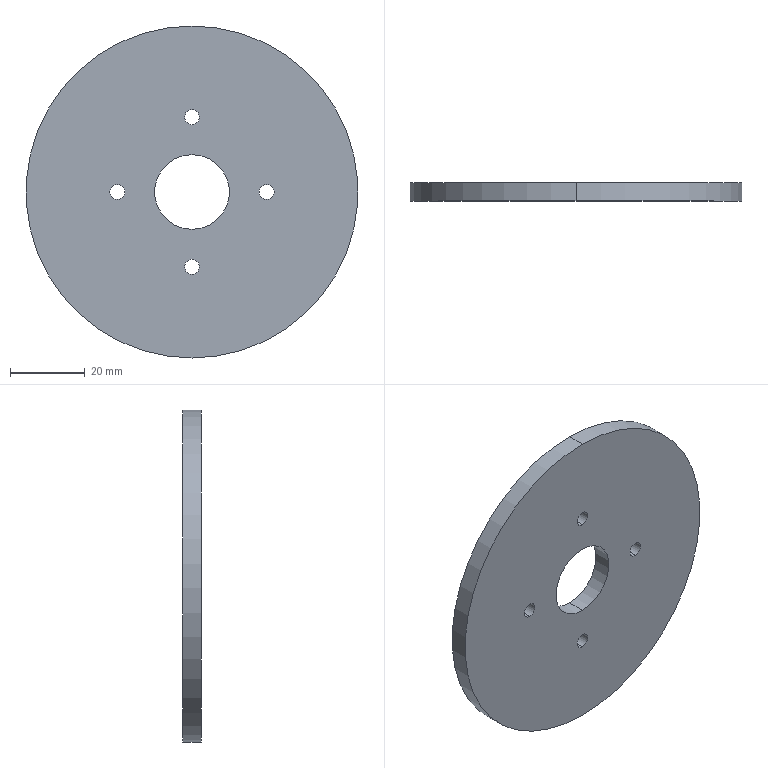Part | STEP file | Guide wheel mechanism revised.sldasm-Part-71 | 1 solid | 34 faces | box 88.8 x 4.9 x 88.8 mm | volume 28486 mm3 | plane 22 | cylinder 12 | commonest cylinder face diameters 4 x8 20 x2 88.8 x2
STEP:
#1=CARTESIAN_POINT('',(-20.,15.1,-2.));
#2=VERTEX_POINT('',#1);
#3=CARTESIAN_POINT('',(-20.,15.1,2.));
#4=VERTEX_POINT('',#3);
#5=CARTESIAN_POINT('',(-20.,15.1,0.));
#6=DIRECTION('',(0.,1.,0.));
#7=DIRECTION('',(0.,0.,-1.));
#8=AXIS2_PLACEMENT_3D('',#5,#6,#7);
#9=CIRCLE('',#8,2.);
#10=EDGE_CURVE('',#2,#4,#9,.T.);
#11=ORIENTED_EDGE('',*,*,#10,.F.);
#12=CARTESIAN_POINT('',(-20.,19.9,-2.));
#13=VERTEX_POINT('',#12);
#14=CARTESIAN_POINT('',(-20.,15.099,-2.));
#15=DIRECTION('',(0.,1.,0.));
#16=VECTOR('',#15,1000.);
#17=LINE('',#14,#16);
#18=EDGE_CURVE('',#2,#13,#17,.T.);
#19=ORIENTED_EDGE('',*,*,#18,.T.);
#20=CARTESIAN_POINT('',(-20.,19.9,2.));
#21=VERTEX_POINT('',#20);
#22=CARTESIAN_POINT('',(-20.,19.9,0.));
#23=DIRECTION('',(0.,1.,0.));
#24=DIRECTION('',(1.,0.,0.));
#25=AXIS2_PLACEMENT_3D('',#22,#23,#24);
#26=CIRCLE('',#25,2.);
#27=EDGE_CURVE('',#13,#21,#26,.T.);
#28=ORIENTED_EDGE('',*,*,#27,.T.);
#29=CARTESIAN_POINT('',(-20.,15.099,2.));
#30=DIRECTION('',(0.,1.,0.));
#31=VECTOR('',#30,1000.);
#32=LINE('',#29,#31);
#33=EDGE_CURVE('',#4,#21,#32,.T.);
#34=ORIENTED_EDGE('',*,*,#33,.F.);
#35=EDGE_LOOP('',(#11,#19,#28,#34));
#36=FACE_OUTER_BOUND('',#35,.T.);
#37=CARTESIAN_POINT('',(-20.,15.099,0.));
#38=DIRECTION('',(0.,1.,0.));
#39=DIRECTION('',(0.,0.,1.));
#40=AXIS2_PLACEMENT_3D('',#37,#38,#39);
#41=CYLINDRICAL_SURFACE('',#40,2.);
#42=ADVANCED_FACE('',(#36),#41,.F.);
#43=CARTESIAN_POINT('',(0.,15.1,18.));
#44=VERTEX_POINT('',#43);
#45=CARTESIAN_POINT('',(0.,15.1,22.));
#46=VERTEX_POINT('',#45);
#47=CARTESIAN_POINT('',(0.,15.1,20.));
#48=DIRECTION('',(0.,1.,0.));
#49=DIRECTION('',(0.,0.,-1.));
#50=AXIS2_PLACEMENT_3D('',#47,#48,#49);
#51=CIRCLE('',#50,2.);
#52=EDGE_CURVE('',#44,#46,#51,.T.);
#53=ORIENTED_EDGE('',*,*,#52,.F.);
#54=CARTESIAN_POINT('',(0.,19.9,18.));
#55=VERTEX_POINT('',#54);
#56=CARTESIAN_POINT('',(0.,15.099,18.));
#57=DIRECTION('',(0.,1.,0.));
#58=VECTOR('',#57,1000.);
#59=LINE('',#56,#58);
#60=EDGE_CURVE('',#44,#55,#59,.T.);
#61=ORIENTED_EDGE('',*,*,#60,.T.);
#62=CARTESIAN_POINT('',(0.,19.9,22.));
#63=VERTEX_POINT('',#62);
#64=CARTESIAN_POINT('',(0.,19.9,20.));
#65=DIRECTION('',(0.,1.,0.));
#66=DIRECTION('',(0.,0.,-1.));
#67=AXIS2_PLACEMENT_3D('',#64,#65,#66);
#68=CIRCLE('',#67,2.);
#69=EDGE_CURVE('',#55,#63,#68,.T.);
#70=ORIENTED_EDGE('',*,*,#69,.T.);
#71=CARTESIAN_POINT('',(0.,15.099,22.));
#72=DIRECTION('',(0.,1.,0.));
#73=VECTOR('',#72,1000.);
#74=LINE('',#71,#73);
#75=EDGE_CURVE('',#46,#63,#74,.T.);
#76=ORIENTED_EDGE('',*,*,#75,.F.);
#77=EDGE_LOOP('',(#53,#61,#70,#76));
#78=FACE_OUTER_BOUND('',#77,.T.);
#79=CARTESIAN_POINT('',(0.,15.099,20.));
#80=DIRECTION('',(0.,1.,0.));
#81=DIRECTION('',(0.,0.,1.));
#82=AXIS2_PLACEMENT_3D('',#79,#80,#81);
#83=CYLINDRICAL_SURFACE('',#82,2.);
#84=ADVANCED_FACE('',(#78),#83,.F.);
#85=CARTESIAN_POINT('',(20.,15.1,-2.));
#86=VERTEX_POINT('',#85);
#87=CARTESIAN_POINT('',(20.,15.1,2.));
#88=VERTEX_POINT('',#87);
#89=CARTESIAN_POINT('',(20.,15.1,0.));
#90=DIRECTION('',(0.,1.,0.));
#91=DIRECTION('',(0.,0.,-1.));
#92=AXIS2_PLACEMENT_3D('',#89,#90,#91);
#93=CIRCLE('',#92,2.);
#94=EDGE_CURVE('',#86,#88,#93,.T.);
#95=ORIENTED_EDGE('',*,*,#94,.F.);
#96=CARTESIAN_POINT('',(20.,19.9,-2.));
#97=VERTEX_POINT('',#96);
#98=CARTESIAN_POINT('',(20.,15.099,-2.));
#99=DIRECTION('',(0.,1.,0.));
#100=VECTOR('',#99,1000.);
#101=LINE('',#98,#100);
#102=EDGE_CURVE('',#86,#97,#101,.T.);
#103=ORIENTED_EDGE('',*,*,#102,.T.);
#104=CARTESIAN_POINT('',(20.,19.9,2.));
#105=VERTEX_POINT('',#104);
#106=CARTESIAN_POINT('',(20.,19.9,0.));
#107=DIRECTION('',(0.,1.,0.));
#108=DIRECTION('',(-1.,0.,0.));
#109=AXIS2_PLACEMENT_3D('',#106,#107,#108);
#110=CIRCLE('',#109,2.);
#111=EDGE_CURVE('',#97,#105,#110,.T.);
#112=ORIENTED_EDGE('',*,*,#111,.T.);
#113=CARTESIAN_POINT('',(20.,15.099,2.));
#114=DIRECTION('',(0.,1.,0.));
#115=VECTOR('',#114,1000.);
#116=LINE('',#113,#115);
#117=EDGE_CURVE('',#88,#105,#116,.T.);
#118=ORIENTED_EDGE('',*,*,#117,.F.);
#119=EDGE_LOOP('',(#95,#103,#112,#118));
#120=FACE_OUTER_BOUND('',#119,.T.);
#121=CARTESIAN_POINT('',(20.,15.099,0.));
#122=DIRECTION('',(0.,1.,0.));
#123=DIRECTION('',(0.,0.,1.));
#124=AXIS2_PLACEMENT_3D('',#121,#122,#123);
#125=CYLINDRICAL_SURFACE('',#124,2.);
#126=ADVANCED_FACE('',(#120),#125,.F.);
#127=CARTESIAN_POINT('',(0.,15.1,-22.));
#128=VERTEX_POINT('',#127);
#129=CARTESIAN_POINT('',(0.,15.1,-18.));
#130=VERTEX_POINT('',#129);
#131=CARTESIAN_POINT('',(0.,15.1,-20.));
#132=DIRECTION('',(0.,1.,0.));
#133=DIRECTION('',(0.,0.,-1.));
#134=AXIS2_PLACEMENT_3D('',#131,#132,#133);
#135=CIRCLE('',#134,2.);
#136=EDGE_CURVE('',#128,#130,#135,.T.);
#137=ORIENTED_EDGE('',*,*,#136,.F.);
#138=CARTESIAN_POINT('',(0.,19.9,-22.));
#139=VERTEX_POINT('',#138);
#140=CARTESIAN_POINT('',(0.,15.099,-22.));
#141=DIRECTION('',(0.,1.,0.));
#142=VECTOR('',#141,1000.);
#143=LINE('',#140,#142);
#144=EDGE_CURVE('',#128,#139,#143,.T.);
#145=ORIENTED_EDGE('',*,*,#144,.T.);
#146=CARTESIAN_POINT('',(0.,19.9,-18.));
#147=VERTEX_POINT('',#146);
#148=CARTESIAN_POINT('',(0.,19.9,-20.));
#149=DIRECTION('',(0.,1.,0.));
#150=DIRECTION('',(0.,0.,1.));
#151=AXIS2_PLACEMENT_3D('',#148,#149,#150);
#152=CIRCLE('',#151,2.);
#153=EDGE_CURVE('',#139,#147,#152,.T.);
#154=ORIENTED_EDGE('',*,*,#153,.T.);
#155=CARTESIAN_POINT('',(0.,15.099,-18.));
#156=DIRECTION('',(0.,1.,0.));
#157=VECTOR('',#156,1000.);
#158=LINE('',#155,#157);
#159=EDGE_CURVE('',#130,#147,#158,.T.);
#160=ORIENTED_EDGE('',*,*,#159,.F.);
#161=EDGE_LOOP('',(#137,#145,#154,#160));
#162=FACE_OUTER_BOUND('',#161,.T.);
#163=CARTESIAN_POINT('',(0.,15.099,-20.));
#164=DIRECTION('',(0.,1.,0.));
#165=DIRECTION('',(0.,0.,1.));
#166=AXIS2_PLACEMENT_3D('',#163,#164,#165);
#167=CYLINDRICAL_SURFACE('',#166,2.);
#168=ADVANCED_FACE('',(#162),#167,.F.);
#169=CARTESIAN_POINT('',(0.,20.,10.));
#170=VERTEX_POINT('',#169);
#171=CARTESIAN_POINT('',(0.,20.,-10.));
#172=VERTEX_POINT('',#171);
#173=CARTESIAN_POINT('',(0.,20.,0.));
#174=DIRECTION('',(0.,-1.,0.));
#175=DIRECTION('',(0.,0.,-1.));
#176=AXIS2_PLACEMENT_3D('',#173,#174,#175);
#177=CIRCLE('',#176,10.);
#178=EDGE_CURVE('',#170,#172,#177,.T.);
#179=ORIENTED_EDGE('',*,*,#178,.F.);
#180=CARTESIAN_POINT('',(0.,15.1,10.));
#181=VERTEX_POINT('',#180);
#182=CARTESIAN_POINT('',(0.,0.,10.));
#183=DIRECTION('',(0.,-1.,0.));
#184=VECTOR('',#183,1000.);
#185=LINE('',#182,#184);
#186=EDGE_CURVE('',#170,#181,#185,.T.);
#187=ORIENTED_EDGE('',*,*,#186,.T.);
#188=CARTESIAN_POINT('',(0.,15.1,-10.));
#189=VERTEX_POINT('',#188);
#190=CARTESIAN_POINT('',(0.,15.1,0.));
#191=DIRECTION('',(0.,-1.,0.));
#192=DIRECTION('',(0.,0.,-1.));
#193=AXIS2_PLACEMENT_3D('',#190,#191,#192);
#194=CIRCLE('',#193,10.);
#195=EDGE_CURVE('',#181,#189,#194,.T.);
#196=ORIENTED_EDGE('',*,*,#195,.T.);
#197=CARTESIAN_POINT('',(0.,0.,-10.));
#198=DIRECTION('',(0.,-1.,0.));
#199=VECTOR('',#198,1000.);
#200=LINE('',#197,#199);
#201=EDGE_CURVE('',#172,#189,#200,.T.);
#202=ORIENTED_EDGE('',*,*,#201,.F.);
#203=EDGE_LOOP('',(#179,#187,#196,#202));
#204=FACE_OUTER_BOUND('',#203,.T.);
#205=CARTESIAN_POINT('',(0.,0.,0.));
#206=DIRECTION('',(0.,-1.,0.));
#207=DIRECTION('',(0.,0.,-1.));
#208=AXIS2_PLACEMENT_3D('',#205,#206,#207);
#209=CYLINDRICAL_SURFACE('',#208,10.);
#210=ADVANCED_FACE('',(#204),#209,.F.);
#211=CARTESIAN_POINT('',(0.,20.,-44.4));
#212=VERTEX_POINT('',#211);
#213=CARTESIAN_POINT('',(0.,20.,44.4));
#214=VERTEX_POINT('',#213);
#215=CARTESIAN_POINT('',(0.,20.,0.));
#216=DIRECTION('',(0.,-1.,0.));
#217=DIRECTION('',(0.,0.,-1.));
#218=AXIS2_PLACEMENT_3D('',#215,#216,#217);
#219=CIRCLE('',#218,44.4);
#220=EDGE_CURVE('',#212,#214,#219,.T.);
#221=ORIENTED_EDGE('',*,*,#220,.T.);
#222=CARTESIAN_POINT('',(0.,15.1,44.4));
#223=VERTEX_POINT('',#222);
#224=CARTESIAN_POINT('',(0.,0.,44.4));
#225=DIRECTION('',(0.,-1.,0.));
#226=VECTOR('',#225,1000.);
#227=LINE('',#224,#226);
#228=EDGE_CURVE('',#214,#223,#227,.T.);
#229=ORIENTED_EDGE('',*,*,#228,.T.);
#230=CARTESIAN_POINT('',(0.,15.1,-44.4));
#231=VERTEX_POINT('',#230);
#232=CARTESIAN_POINT('',(0.,15.1,0.));
#233=DIRECTION('',(0.,-1.,0.));
#234=DIRECTION('',(0.,0.,-1.));
#235=AXIS2_PLACEMENT_3D('',#232,#233,#234);
#236=CIRCLE('',#235,44.4);
#237=EDGE_CURVE('',#231,#223,#236,.T.);
#238=ORIENTED_EDGE('',*,*,#237,.F.);
#239=CARTESIAN_POINT('',(0.,0.,-44.4));
#240=DIRECTION('',(0.,-1.,0.));
#241=VECTOR('',#240,1000.);
#242=LINE('',#239,#241);
#243=EDGE_CURVE('',#212,#231,#242,.T.);
#244=ORIENTED_EDGE('',*,*,#243,.F.);
#245=EDGE_LOOP('',(#221,#229,#238,#244));
#246=FACE_OUTER_BOUND('',#245,.T.);
#247=CARTESIAN_POINT('',(0.,0.,0.));
#248=DIRECTION('',(0.,-1.,0.));
#249=DIRECTION('',(0.,0.,-1.));
#250=AXIS2_PLACEMENT_3D('',#247,#248,#249);
#251=CYLINDRICAL_SURFACE('',#250,44.4);
#252=ADVANCED_FACE('',(#246),#251,.T.);
#253=ORIENTED_EDGE('',*,*,#228,.F.);
#254=CARTESIAN_POINT('',(0.,20.,0.));
#255=DIRECTION('',(0.,-1.,0.));
#256=DIRECTION('',(0.,0.,-1.));
#257=AXIS2_PLACEMENT_3D('',#254,#255,#256);
#258=CIRCLE('',#257,44.4);
#259=EDGE_CURVE('',#214,#212,#258,.T.);
#260=ORIENTED_EDGE('',*,*,#259,.T.);
#261=ORIENTED_EDGE('',*,*,#243,.T.);
#262=CARTESIAN_POINT('',(0.,15.1,0.));
#263=DIRECTION('',(0.,-1.,0.));
#264=DIRECTION('',(0.,0.,-1.));
#265=AXIS2_PLACEMENT_3D('',#262,#263,#264);
#266=CIRCLE('',#265,44.4);
#267=EDGE_CURVE('',#223,#231,#266,.T.);
#268=ORIENTED_EDGE('',*,*,#267,.F.);
#269=EDGE_LOOP('',(#253,#260,#261,#268));
#270=FACE_OUTER_BOUND('',#269,.T.);
#271=CARTESIAN_POINT('',(0.,0.,0.));
#272=DIRECTION('',(0.,-1.,0.));
#273=DIRECTION('',(0.,0.,-1.));
#274=AXIS2_PLACEMENT_3D('',#271,#272,#273);
#275=CYLINDRICAL_SURFACE('',#274,44.4);
#276=ADVANCED_FACE('',(#270),#275,.T.);
#277=CARTESIAN_POINT('',(-35.,20.,5.));
#278=VERTEX_POINT('',#277);
#279=CARTESIAN_POINT('',(-15.,20.,5.));
#280=VERTEX_POINT('',#279);
#281=CARTESIAN_POINT('',(-35.,20.,5.));
#282=DIRECTION('',(1.,0.,0.));
#283=VECTOR('',#282,1000.);
#284=LINE('',#281,#283);
#285=EDGE_CURVE('',#278,#280,#284,.T.);
#286=ORIENTED_EDGE('',*,*,#285,.F.);
#287=CARTESIAN_POINT('',(-35.,20.,-5.));
#288=VERTEX_POINT('',#287);
#289=CARTESIAN_POINT('',(-35.,20.,5.));
#290=DIRECTION('',(0.,0.,1.));
#291=VECTOR('',#290,1000.);
#292=LINE('',#289,#291);
#293=EDGE_CURVE('',#288,#278,#292,.T.);
#294=ORIENTED_EDGE('',*,*,#293,.F.);
#295=CARTESIAN_POINT('',(-15.,20.,-5.));
#296=VERTEX_POINT('',#295);
#297=CARTESIAN_POINT('',(-35.,20.,-5.));
#298=DIRECTION('',(-1.,0.,0.));
#299=VECTOR('',#298,1000.);
#300=LINE('',#297,#299);
#301=EDGE_CURVE('',#296,#288,#300,.T.);
#302=ORIENTED_EDGE('',*,*,#301,.F.);
#303=CARTESIAN_POINT('',(-15.,20.,5.));
#304=DIRECTION('',(0.,0.,-1.));
#305=VECTOR('',#304,1000.);
#306=LINE('',#303,#305);
#307=EDGE_CURVE('',#280,#296,#306,.T.);
#308=ORIENTED_EDGE('',*,*,#307,.F.);
#309=EDGE_LOOP('',(#286,#294,#302,#308));
#310=FACE_BOUND('',#309,.T.);
#311=CARTESIAN_POINT('',(5.,20.,35.));
#312=VERTEX_POINT('',#311);
#313=CARTESIAN_POINT('',(5.,20.,15.));
#314=VERTEX_POINT('',#313);
#315=CARTESIAN_POINT('',(5.,20.,35.));
#316=DIRECTION('',(0.,0.,-1.));
#317=VECTOR('',#316,1000.);
#318=LINE('',#315,#317);
#319=EDGE_CURVE('',#312,#314,#318,.T.);
#320=ORIENTED_EDGE('',*,*,#319,.F.);
#321=CARTESIAN_POINT('',(-5.,20.,35.));
#322=VERTEX_POINT('',#321);
#323=CARTESIAN_POINT('',(5.,20.,35.));
#324=DIRECTION('',(1.,0.,0.));
#325=VECTOR('',#324,1000.);
#326=LINE('',#323,#325);
#327=EDGE_CURVE('',#322,#312,#326,.T.);
#328=ORIENTED_EDGE('',*,*,#327,.F.);
#329=CARTESIAN_POINT('',(-5.,20.,15.));
#330=VERTEX_POINT('',#329);
#331=CARTESIAN_POINT('',(-5.,20.,35.));
#332=DIRECTION('',(0.,0.,1.));
#333=VECTOR('',#332,1000.);
#334=LINE('',#331,#333);
#335=EDGE_CURVE('',#330,#322,#334,.T.);
#336=ORIENTED_EDGE('',*,*,#335,.F.);
#337=CARTESIAN_POINT('',(5.,20.,15.));
#338=DIRECTION('',(-1.,0.,0.));
#339=VECTOR('',#338,1000.);
#340=LINE('',#337,#339);
#341=EDGE_CURVE('',#314,#330,#340,.T.);
#342=ORIENTED_EDGE('',*,*,#341,.F.);
#343=EDGE_LOOP('',(#320,#328,#336,#342));
#344=FACE_BOUND('',#343,.T.);
#345=CARTESIAN_POINT('',(35.,20.,-5.));
#346=VERTEX_POINT('',#345);
#347=CARTESIAN_POINT('',(15.,20.,-5.));
#348=VERTEX_POINT('',#347);
#349=CARTESIAN_POINT('',(35.,20.,-5.));
#350=DIRECTION('',(-1.,0.,0.));
#351=VECTOR('',#350,1000.);
#352=LINE('',#349,#351);
#353=EDGE_CURVE('',#346,#348,#352,.T.);
#354=ORIENTED_EDGE('',*,*,#353,.F.);
#355=CARTESIAN_POINT('',(35.,20.,5.));
#356=VERTEX_POINT('',#355);
#357=CARTESIAN_POINT('',(35.,20.,-5.));
#358=DIRECTION('',(0.,0.,-1.));
#359=VECTOR('',#358,1000.);
#360=LINE('',#357,#359);
#361=EDGE_CURVE('',#356,#346,#360,.T.);
#362=ORIENTED_EDGE('',*,*,#361,.F.);
#363=CARTESIAN_POINT('',(15.,20.,5.));
#364=VERTEX_POINT('',#363);
#365=CARTESIAN_POINT('',(35.,20.,5.));
#366=DIRECTION('',(1.,0.,0.));
#367=VECTOR('',#366,1000.);
#368=LINE('',#365,#367);
#369=EDGE_CURVE('',#364,#356,#368,.T.);
#370=ORIENTED_EDGE('',*,*,#369,.F.);
#371=CARTESIAN_POINT('',(15.,20.,-5.));
#372=DIRECTION('',(0.,0.,1.));
#373=VECTOR('',#372,1000.);
#374=LINE('',#371,#373);
#375=EDGE_CURVE('',#348,#364,#374,.T.);
#376=ORIENTED_EDGE('',*,*,#375,.F.);
#377=EDGE_LOOP('',(#354,#362,#370,#376));
#378=FACE_BOUND('',#377,.T.);
#379=CARTESIAN_POINT('',(-5.,20.,-35.));
#380=VERTEX_POINT('',#379);
#381=CARTESIAN_POINT('',(-5.,20.,-15.));
#382=VERTEX_POINT('',#381);
#383=CARTESIAN_POINT('',(-5.,20.,-35.));
#384=DIRECTION('',(0.,0.,1.));
#385=VECTOR('',#384,1000.);
#386=LINE('',#383,#385);
#387=EDGE_CURVE('',#380,#382,#386,.T.);
#388=ORIENTED_EDGE('',*,*,#387,.F.);
#389=CARTESIAN_POINT('',(5.,20.,-35.));
#390=VERTEX_POINT('',#389);
#391=CARTESIAN_POINT('',(-5.,20.,-35.));
#392=DIRECTION('',(-1.,0.,0.));
#393=VECTOR('',#392,1000.);
#394=LINE('',#391,#393);
#395=EDGE_CURVE('',#390,#380,#394,.T.);
#396=ORIENTED_EDGE('',*,*,#395,.F.);
#397=CARTESIAN_POINT('',(5.,20.,-15.));
#398=VERTEX_POINT('',#397);
#399=CARTESIAN_POINT('',(5.,20.,-35.));
#400=DIRECTION('',(0.,0.,-1.));
#401=VECTOR('',#400,1000.);
#402=LINE('',#399,#401);
#403=EDGE_CURVE('',#398,#390,#402,.T.);
#404=ORIENTED_EDGE('',*,*,#403,.F.);
#405=CARTESIAN_POINT('',(-5.,20.,-15.));
#406=DIRECTION('',(1.,0.,0.));
#407=VECTOR('',#406,1000.);
#408=LINE('',#405,#407);
#409=EDGE_CURVE('',#382,#398,#408,.T.);
#410=ORIENTED_EDGE('',*,*,#409,.F.);
#411=EDGE_LOOP('',(#388,#396,#404,#410));
#412=FACE_BOUND('',#411,.T.);
#413=CARTESIAN_POINT('',(0.,20.,0.));
#414=DIRECTION('',(0.,-1.,0.));
#415=DIRECTION('',(0.,0.,-1.));
#416=AXIS2_PLACEMENT_3D('',#413,#414,#415);
#417=CIRCLE('',#416,10.);
#418=EDGE_CURVE('',#172,#170,#417,.T.);
#419=ORIENTED_EDGE('',*,*,#418,.T.);
#420=ORIENTED_EDGE('',*,*,#178,.T.);
#421=EDGE_LOOP('',(#419,#420));
#422=FACE_BOUND('',#421,.T.);
#423=ORIENTED_EDGE('',*,*,#220,.F.);
#424=ORIENTED_EDGE('',*,*,#259,.F.);
#425=EDGE_LOOP('',(#423,#424));
#426=FACE_OUTER_BOUND('',#425,.T.);
#427=CARTESIAN_POINT('',(44.4,20.,0.));
#428=DIRECTION('',(0.,1.,0.));
#429=DIRECTION('',(0.,0.,1.));
#430=AXIS2_PLACEMENT_3D('',#427,#428,#429);
#431=PLANE('',#430);
#432=ADVANCED_FACE('',(#310,#344,#378,#412,#422,#426),#431,.T.);
#433=ORIENTED_EDGE('',*,*,#186,.F.);
#434=ORIENTED_EDGE('',*,*,#418,.F.);
#435=ORIENTED_EDGE('',*,*,#201,.T.);
#436=CARTESIAN_POINT('',(0.,15.1,0.));
#437=DIRECTION('',(0.,-1.,0.));
#438=DIRECTION('',(0.,0.,-1.));
#439=AXIS2_PLACEMENT_3D('',#436,#437,#438);
#440=CIRCLE('',#439,10.);
#441=EDGE_CURVE('',#189,#181,#440,.T.);
#442=ORIENTED_EDGE('',*,*,#441,.T.);
#443=EDGE_LOOP('',(#433,#434,#435,#442));
#444=FACE_OUTER_BOUND('',#443,.T.);
#445=CARTESIAN_POINT('',(0.,0.,0.));
#446=DIRECTION('',(0.,-1.,0.));
#447=DIRECTION('',(0.,0.,-1.));
#448=AXIS2_PLACEMENT_3D('',#445,#446,#447);
#449=CYLINDRICAL_SURFACE('',#448,10.);
#450=ADVANCED_FACE('',(#444),#449,.F.);
#451=CARTESIAN_POINT('',(-20.,15.1,0.));
#452=DIRECTION('',(0.,1.,0.));
#453=DIRECTION('',(0.,0.,-1.));
#454=AXIS2_PLACEMENT_3D('',#451,#452,#453);
#455=CIRCLE('',#454,2.);
#456=EDGE_CURVE('',#4,#2,#455,.T.);
#457=ORIENTED_EDGE('',*,*,#456,.T.);
#458=ORIENTED_EDGE('',*,*,#10,.T.);
#459=EDGE_LOOP('',(#457,#458));
#460=FACE_BOUND('',#459,.T.);
#461=CARTESIAN_POINT('',(0.,15.1,20.));
#462=DIRECTION('',(0.,1.,0.));
#463=DIRECTION('',(0.,0.,-1.));
#464=AXIS2_PLACEMENT_3D('',#461,#462,#463);
#465=CIRCLE('',#464,2.);
#466=EDGE_CURVE('',#46,#44,#465,.T.);
#467=ORIENTED_EDGE('',*,*,#466,.T.);
#468=ORIENTED_EDGE('',*,*,#52,.T.);
#469=EDGE_LOOP('',(#467,#468));
#470=FACE_BOUND('',#469,.T.);
#471=CARTESIAN_POINT('',(20.,15.1,0.));
#472=DIRECTION('',(0.,1.,0.));
#473=DIRECTION('',(0.,0.,-1.));
#474=AXIS2_PLACEMENT_3D('',#471,#472,#473);
#475=CIRCLE('',#474,2.);
#476=EDGE_CURVE('',#88,#86,#475,.T.);
#477=ORIENTED_EDGE('',*,*,#476,.T.);
#478=ORIENTED_EDGE('',*,*,#94,.T.);
#479=EDGE_LOOP('',(#477,#478));
#480=FACE_BOUND('',#479,.T.);
#481=CARTESIAN_POINT('',(0.,15.1,-20.));
#482=DIRECTION('',(0.,1.,0.));
#483=DIRECTION('',(0.,0.,-1.));
#484=AXIS2_PLACEMENT_3D('',#481,#482,#483);
#485=CIRCLE('',#484,2.);
#486=EDGE_CURVE('',#130,#128,#485,.T.);
#487=ORIENTED_EDGE('',*,*,#486,.T.);
#488=ORIENTED_EDGE('',*,*,#136,.T.);
#489=EDGE_LOOP('',(#487,#488));
#490=FACE_BOUND('',#489,.T.);
#491=ORIENTED_EDGE('',*,*,#237,.T.);
#492=ORIENTED_EDGE('',*,*,#267,.T.);
#493=EDGE_LOOP('',(#491,#492));
#494=FACE_OUTER_BOUND('',#493,.T.);
#495=ORIENTED_EDGE('',*,*,#441,.F.);
#496=ORIENTED_EDGE('',*,*,#195,.F.);
#497=EDGE_LOOP('',(#495,#496));
#498=FACE_BOUND('',#497,.T.);
#499=CARTESIAN_POINT('',(10.,15.1,0.));
#500=DIRECTION('',(0.,-1.,0.));
#501=DIRECTION('',(0.,0.,-1.));
#502=AXIS2_PLACEMENT_3D('',#499,#500,#501);
#503=PLANE('',#502);
#504=ADVANCED_FACE('',(#460,#470,#480,#490,#494,#498),#503,.T.);
#505=ORIENTED_EDGE('',*,*,#387,.T.);
#506=CARTESIAN_POINT('',(-5.,19.9,-15.));
#507=VERTEX_POINT('',#506);
#508=CARTESIAN_POINT('',(-5.,19.9,-15.));
#509=DIRECTION('',(0.,1.,0.));
#510=VECTOR('',#509,1000.);
#511=LINE('',#508,#510);
#512=EDGE_CURVE('',#507,#382,#511,.T.);
#513=ORIENTED_EDGE('',*,*,#512,.F.);
#514=CARTESIAN_POINT('',(-5.,19.9,-35.));
#515=VERTEX_POINT('',#514);
#516=CARTESIAN_POINT('',(-5.,19.9,-35.));
#517=DIRECTION('',(0.,0.,1.));
#518=VECTOR('',#517,1000.);
#519=LINE('',#516,#518);
#520=EDGE_CURVE('',#515,#507,#519,.T.);
#521=ORIENTED_EDGE('',*,*,#520,.F.);
#522=CARTESIAN_POINT('',(-5.,19.9,-35.));
#523=DIRECTION('',(0.,1.,0.));
#524=VECTOR('',#523,1000.);
#525=LINE('',#522,#524);
#526=EDGE_CURVE('',#515,#380,#525,.T.);
#527=ORIENTED_EDGE('',*,*,#526,.T.);
#528=EDGE_LOOP('',(#505,#513,#521,#527));
#529=FACE_OUTER_BOUND('',#528,.T.);
#530=CARTESIAN_POINT('',(-5.,19.9,-35.));
#531=DIRECTION('',(-1.,0.,0.));
#532=DIRECTION('',(0.,0.,1.));
#533=AXIS2_PLACEMENT_3D('',#530,#531,#532);
#534=PLANE('',#533);
#535=ADVANCED_FACE('',(#529),#534,.F.);
#536=ORIENTED_EDGE('',*,*,#395,.T.);
#537=ORIENTED_EDGE('',*,*,#526,.F.);
#538=CARTESIAN_POINT('',(5.,19.9,-35.));
#539=VERTEX_POINT('',#538);
#540=CARTESIAN_POINT('',(-5.,19.9,-35.));
#541=DIRECTION('',(-1.,0.,0.));
#542=VECTOR('',#541,1000.);
#543=LINE('',#540,#542);
#544=EDGE_CURVE('',#539,#515,#543,.T.);
#545=ORIENTED_EDGE('',*,*,#544,.F.);
#546=CARTESIAN_POINT('',(5.,19.9,-35.));
#547=DIRECTION('',(0.,1.,0.));
#548=VECTOR('',#547,1000.);
#549=LINE('',#546,#548);
#550=EDGE_CURVE('',#539,#390,#549,.T.);
#551=ORIENTED_EDGE('',*,*,#550,.T.);
#552=EDGE_LOOP('',(#536,#537,#545,#551));
#553=FACE_OUTER_BOUND('',#552,.T.);
#554=CARTESIAN_POINT('',(-5.,19.9,-35.));
#555=DIRECTION('',(0.,0.,-1.));
#556=DIRECTION('',(-1.,0.,0.));
#557=AXIS2_PLACEMENT_3D('',#554,#555,#556);
#558=PLANE('',#557);
#559=ADVANCED_FACE('',(#553),#558,.F.);
#560=ORIENTED_EDGE('',*,*,#403,.T.);
#561=ORIENTED_EDGE('',*,*,#550,.F.);
#562=CARTESIAN_POINT('',(5.,19.9,-15.));
#563=VERTEX_POINT('',#562);
#564=CARTESIAN_POINT('',(5.,19.9,-35.));
#565=DIRECTION('',(0.,0.,-1.));
#566=VECTOR('',#565,1000.);
#567=LINE('',#564,#566);
#568=EDGE_CURVE('',#563,#539,#567,.T.);
#569=ORIENTED_EDGE('',*,*,#568,.F.);
#570=CARTESIAN_POINT('',(5.,19.9,-15.));
#571=DIRECTION('',(0.,1.,0.));
#572=VECTOR('',#571,1000.);
#573=LINE('',#570,#572);
#574=EDGE_CURVE('',#563,#398,#573,.T.);
#575=ORIENTED_EDGE('',*,*,#574,.T.);
#576=EDGE_LOOP('',(#560,#561,#569,#575));
#577=FACE_OUTER_BOUND('',#576,.T.);
#578=CARTESIAN_POINT('',(5.,19.9,-35.));
#579=DIRECTION('',(1.,0.,0.));
#580=DIRECTION('',(0.,0.,-1.));
#581=AXIS2_PLACEMENT_3D('',#578,#579,#580);
#582=PLANE('',#581);
#583=ADVANCED_FACE('',(#577),#582,.F.);
#584=ORIENTED_EDGE('',*,*,#409,.T.);
#585=ORIENTED_EDGE('',*,*,#574,.F.);
#586=CARTESIAN_POINT('',(-5.,19.9,-15.));
#587=DIRECTION('',(1.,0.,0.));
#588=VECTOR('',#587,1000.);
#589=LINE('',#586,#588);
#590=EDGE_CURVE('',#507,#563,#589,.T.);
#591=ORIENTED_EDGE('',*,*,#590,.F.);
#592=ORIENTED_EDGE('',*,*,#512,.T.);
#593=EDGE_LOOP('',(#584,#585,#591,#592));
#594=FACE_OUTER_BOUND('',#593,.T.);
#595=CARTESIAN_POINT('',(-5.,19.9,-15.));
#596=DIRECTION('',(0.,0.,1.));
#597=DIRECTION('',(1.,0.,0.));
#598=AXIS2_PLACEMENT_3D('',#595,#596,#597);
#599=PLANE('',#598);
#600=ADVANCED_FACE('',(#594),#599,.F.);
#601=CARTESIAN_POINT('',(0.,19.9,-20.));
#602=DIRECTION('',(0.,1.,0.));
#603=DIRECTION('',(0.,0.,1.));
#604=AXIS2_PLACEMENT_3D('',#601,#602,#603);
#605=CIRCLE('',#604,2.);
#606=EDGE_CURVE('',#147,#139,#605,.T.);
#607=ORIENTED_EDGE('',*,*,#606,.F.);
#608=ORIENTED_EDGE('',*,*,#153,.F.);
#609=EDGE_LOOP('',(#607,#608));
#610=FACE_BOUND('',#609,.T.);
#611=ORIENTED_EDGE('',*,*,#520,.T.);
#612=ORIENTED_EDGE('',*,*,#590,.T.);
#613=ORIENTED_EDGE('',*,*,#568,.T.);
#614=ORIENTED_EDGE('',*,*,#544,.T.);
#615=EDGE_LOOP('',(#611,#612,#613,#614));
#616=FACE_OUTER_BOUND('',#615,.T.);
#617=CARTESIAN_POINT('',(0.,19.9,0.));
#618=DIRECTION('',(0.,1.,0.));
#619=DIRECTION('',(0.,0.,1.));
#620=AXIS2_PLACEMENT_3D('',#617,#618,#619);
#621=PLANE('',#620);
#622=ADVANCED_FACE('',(#610,#616),#621,.T.);
#623=ORIENTED_EDGE('',*,*,#144,.F.);
#624=ORIENTED_EDGE('',*,*,#486,.F.);
#625=ORIENTED_EDGE('',*,*,#159,.T.);
#626=ORIENTED_EDGE('',*,*,#606,.T.);
#627=EDGE_LOOP('',(#623,#624,#625,#626));
#628=FACE_OUTER_BOUND('',#627,.T.);
#629=CARTESIAN_POINT('',(0.,15.099,-20.));
#630=DIRECTION('',(0.,1.,0.));
#631=DIRECTION('',(0.,0.,1.));
#632=AXIS2_PLACEMENT_3D('',#629,#630,#631);
#633=CYLINDRICAL_SURFACE('',#632,2.);
#634=ADVANCED_FACE('',(#628),#633,.F.);
#635=ORIENTED_EDGE('',*,*,#353,.T.);
#636=CARTESIAN_POINT('',(15.,19.9,-5.));
#637=VERTEX_POINT('',#636);
#638=CARTESIAN_POINT('',(15.,19.9,-5.));
#639=DIRECTION('',(0.,1.,0.));
#640=VECTOR('',#639,1000.);
#641=LINE('',#638,#640);
#642=EDGE_CURVE('',#637,#348,#641,.T.);
#643=ORIENTED_EDGE('',*,*,#642,.F.);
#644=CARTESIAN_POINT('',(35.,19.9,-5.));
#645=VERTEX_POINT('',#644);
#646=CARTESIAN_POINT('',(35.,19.9,-5.));
#647=DIRECTION('',(-1.,0.,0.));
#648=VECTOR('',#647,1000.);
#649=LINE('',#646,#648);
#650=EDGE_CURVE('',#645,#637,#649,.T.);
#651=ORIENTED_EDGE('',*,*,#650,.F.);
#652=CARTESIAN_POINT('',(35.,19.9,-5.));
#653=DIRECTION('',(0.,1.,0.));
#654=VECTOR('',#653,1000.);
#655=LINE('',#652,#654);
#656=EDGE_CURVE('',#645,#346,#655,.T.);
#657=ORIENTED_EDGE('',*,*,#656,.T.);
#658=EDGE_LOOP('',(#635,#643,#651,#657));
#659=FACE_OUTER_BOUND('',#658,.T.);
#660=CARTESIAN_POINT('',(35.,19.9,-5.));
#661=DIRECTION('',(0.,0.,-1.));
#662=DIRECTION('',(-1.,0.,0.));
#663=AXIS2_PLACEMENT_3D('',#660,#661,#662);
#664=PLANE('',#663);
#665=ADVANCED_FACE('',(#659),#664,.F.);
#666=ORIENTED_EDGE('',*,*,#361,.T.);
#667=ORIENTED_EDGE('',*,*,#656,.F.);
#668=CARTESIAN_POINT('',(35.,19.9,5.));
#669=VERTEX_POINT('',#668);
#670=CARTESIAN_POINT('',(35.,19.9,-5.));
#671=DIRECTION('',(0.,0.,-1.));
#672=VECTOR('',#671,1000.);
#673=LINE('',#670,#672);
#674=EDGE_CURVE('',#669,#645,#673,.T.);
#675=ORIENTED_EDGE('',*,*,#674,.F.);
#676=CARTESIAN_POINT('',(35.,19.9,5.));
#677=DIRECTION('',(0.,1.,0.));
#678=VECTOR('',#677,1000.);
#679=LINE('',#676,#678);
#680=EDGE_CURVE('',#669,#356,#679,.T.);
#681=ORIENTED_EDGE('',*,*,#680,.T.);
#682=EDGE_LOOP('',(#666,#667,#675,#681));
#683=FACE_OUTER_BOUND('',#682,.T.);
#684=CARTESIAN_POINT('',(35.,19.9,-5.));
#685=DIRECTION('',(1.,0.,0.));
#686=DIRECTION('',(0.,0.,-1.));
#687=AXIS2_PLACEMENT_3D('',#684,#685,#686);
#688=PLANE('',#687);
#689=ADVANCED_FACE('',(#683),#688,.F.);
#690=ORIENTED_EDGE('',*,*,#369,.T.);
#691=ORIENTED_EDGE('',*,*,#680,.F.);
#692=CARTESIAN_POINT('',(15.,19.9,5.));
#693=VERTEX_POINT('',#692);
#694=CARTESIAN_POINT('',(35.,19.9,5.));
#695=DIRECTION('',(1.,0.,0.));
#696=VECTOR('',#695,1000.);
#697=LINE('',#694,#696);
#698=EDGE_CURVE('',#693,#669,#697,.T.);
#699=ORIENTED_EDGE('',*,*,#698,.F.);
#700=CARTESIAN_POINT('',(15.,19.9,5.));
#701=DIRECTION('',(0.,1.,0.));
#702=VECTOR('',#701,1000.);
#703=LINE('',#700,#702);
#704=EDGE_CURVE('',#693,#364,#703,.T.);
#705=ORIENTED_EDGE('',*,*,#704,.T.);
#706=EDGE_LOOP('',(#690,#691,#699,#705));
#707=FACE_OUTER_BOUND('',#706,.T.);
#708=CARTESIAN_POINT('',(35.,19.9,5.));
#709=DIRECTION('',(0.,0.,1.));
#710=DIRECTION('',(1.,0.,0.));
#711=AXIS2_PLACEMENT_3D('',#708,#709,#710);
#712=PLANE('',#711);
#713=ADVANCED_FACE('',(#707),#712,.F.);
#714=ORIENTED_EDGE('',*,*,#375,.T.);
#715=ORIENTED_EDGE('',*,*,#704,.F.);
#716=CARTESIAN_POINT('',(15.,19.9,-5.));
#717=DIRECTION('',(0.,0.,1.));
#718=VECTOR('',#717,1000.);
#719=LINE('',#716,#718);
#720=EDGE_CURVE('',#637,#693,#719,.T.);
#721=ORIENTED_EDGE('',*,*,#720,.F.);
#722=ORIENTED_EDGE('',*,*,#642,.T.);
#723=EDGE_LOOP('',(#714,#715,#721,#722));
#724=FACE_OUTER_BOUND('',#723,.T.);
#725=CARTESIAN_POINT('',(15.,19.9,-5.));
#726=DIRECTION('',(-1.,0.,0.));
#727=DIRECTION('',(0.,0.,1.));
#728=AXIS2_PLACEMENT_3D('',#725,#726,#727);
#729=PLANE('',#728);
#730=ADVANCED_FACE('',(#724),#729,.F.);
#731=CARTESIAN_POINT('',(20.,19.9,0.));
#732=DIRECTION('',(0.,1.,0.));
#733=DIRECTION('',(-1.,0.,0.));
#734=AXIS2_PLACEMENT_3D('',#731,#732,#733);
#735=CIRCLE('',#734,2.);
#736=EDGE_CURVE('',#105,#97,#735,.T.);
#737=ORIENTED_EDGE('',*,*,#736,.F.);
#738=ORIENTED_EDGE('',*,*,#111,.F.);
#739=EDGE_LOOP('',(#737,#738));
#740=FACE_BOUND('',#739,.T.);
#741=ORIENTED_EDGE('',*,*,#650,.T.);
#742=ORIENTED_EDGE('',*,*,#720,.T.);
#743=ORIENTED_EDGE('',*,*,#698,.T.);
#744=ORIENTED_EDGE('',*,*,#674,.T.);
#745=EDGE_LOOP('',(#741,#742,#743,#744));
#746=FACE_OUTER_BOUND('',#745,.T.);
#747=CARTESIAN_POINT('',(0.,19.9,0.));
#748=DIRECTION('',(0.,1.,0.));
#749=DIRECTION('',(-1.,0.,0.));
#750=AXIS2_PLACEMENT_3D('',#747,#748,#749);
#751=PLANE('',#750);
#752=ADVANCED_FACE('',(#740,#746),#751,.T.);
#753=ORIENTED_EDGE('',*,*,#319,.T.);
#754=CARTESIAN_POINT('',(5.,19.9,15.));
#755=VERTEX_POINT('',#754);
#756=CARTESIAN_POINT('',(5.,19.9,15.));
#757=DIRECTION('',(0.,1.,0.));
#758=VECTOR('',#757,1000.);
#759=LINE('',#756,#758);
#760=EDGE_CURVE('',#755,#314,#759,.T.);
#761=ORIENTED_EDGE('',*,*,#760,.F.);
#762=CARTESIAN_POINT('',(5.,19.9,35.));
#763=VERTEX_POINT('',#762);
#764=CARTESIAN_POINT('',(5.,19.9,35.));
#765=DIRECTION('',(0.,0.,-1.));
#766=VECTOR('',#765,1000.);
#767=LINE('',#764,#766);
#768=EDGE_CURVE('',#763,#755,#767,.T.);
#769=ORIENTED_EDGE('',*,*,#768,.F.);
#770=CARTESIAN_POINT('',(5.,19.9,35.));
#771=DIRECTION('',(0.,1.,0.));
#772=VECTOR('',#771,1000.);
#773=LINE('',#770,#772);
#774=EDGE_CURVE('',#763,#312,#773,.T.);
#775=ORIENTED_EDGE('',*,*,#774,.T.);
#776=EDGE_LOOP('',(#753,#761,#769,#775));
#777=FACE_OUTER_BOUND('',#776,.T.);
#778=CARTESIAN_POINT('',(5.,19.9,35.));
#779=DIRECTION('',(1.,0.,0.));
#780=DIRECTION('',(0.,0.,-1.));
#781=AXIS2_PLACEMENT_3D('',#778,#779,#780);
#782=PLANE('',#781);
#783=ADVANCED_FACE('',(#777),#782,.F.);
#784=ORIENTED_EDGE('',*,*,#327,.T.);
#785=ORIENTED_EDGE('',*,*,#774,.F.);
#786=CARTESIAN_POINT('',(-5.,19.9,35.));
#787=VERTEX_POINT('',#786);
#788=CARTESIAN_POINT('',(5.,19.9,35.));
#789=DIRECTION('',(1.,0.,0.));
#790=VECTOR('',#789,1000.);
#791=LINE('',#788,#790);
#792=EDGE_CURVE('',#787,#763,#791,.T.);
#793=ORIENTED_EDGE('',*,*,#792,.F.);
#794=CARTESIAN_POINT('',(-5.,19.9,35.));
#795=DIRECTION('',(0.,1.,0.));
#796=VECTOR('',#795,1000.);
#797=LINE('',#794,#796);
#798=EDGE_CURVE('',#787,#322,#797,.T.);
#799=ORIENTED_EDGE('',*,*,#798,.T.);
#800=EDGE_LOOP('',(#784,#785,#793,#799));
#801=FACE_OUTER_BOUND('',#800,.T.);
#802=CARTESIAN_POINT('',(5.,19.9,35.));
#803=DIRECTION('',(0.,0.,1.));
#804=DIRECTION('',(1.,0.,0.));
#805=AXIS2_PLACEMENT_3D('',#802,#803,#804);
#806=PLANE('',#805);
#807=ADVANCED_FACE('',(#801),#806,.F.);
#808=ORIENTED_EDGE('',*,*,#335,.T.);
#809=ORIENTED_EDGE('',*,*,#798,.F.);
#810=CARTESIAN_POINT('',(-5.,19.9,15.));
#811=VERTEX_POINT('',#810);
#812=CARTESIAN_POINT('',(-5.,19.9,35.));
#813=DIRECTION('',(0.,0.,1.));
#814=VECTOR('',#813,1000.);
#815=LINE('',#812,#814);
#816=EDGE_CURVE('',#811,#787,#815,.T.);
#817=ORIENTED_EDGE('',*,*,#816,.F.);
#818=CARTESIAN_POINT('',(-5.,19.9,15.));
#819=DIRECTION('',(0.,1.,0.));
#820=VECTOR('',#819,1000.);
#821=LINE('',#818,#820);
#822=EDGE_CURVE('',#811,#330,#821,.T.);
#823=ORIENTED_EDGE('',*,*,#822,.T.);
#824=EDGE_LOOP('',(#808,#809,#817,#823));
#825=FACE_OUTER_BOUND('',#824,.T.);
#826=CARTESIAN_POINT('',(-5.,19.9,35.));
#827=DIRECTION('',(-1.,0.,0.));
#828=DIRECTION('',(0.,0.,1.));
#829=AXIS2_PLACEMENT_3D('',#826,#827,#828);
#830=PLANE('',#829);
#831=ADVANCED_FACE('',(#825),#830,.F.);
#832=ORIENTED_EDGE('',*,*,#341,.T.);
#833=ORIENTED_EDGE('',*,*,#822,.F.);
#834=CARTESIAN_POINT('',(5.,19.9,15.));
#835=DIRECTION('',(-1.,0.,0.));
#836=VECTOR('',#835,1000.);
#837=LINE('',#834,#836);
#838=EDGE_CURVE('',#755,#811,#837,.T.);
#839=ORIENTED_EDGE('',*,*,#838,.F.);
#840=ORIENTED_EDGE('',*,*,#760,.T.);
#841=EDGE_LOOP('',(#832,#833,#839,#840));
#842=FACE_OUTER_BOUND('',#841,.T.);
#843=CARTESIAN_POINT('',(5.,19.9,15.));
#844=DIRECTION('',(0.,0.,-1.));
#845=DIRECTION('',(-1.,0.,0.));
#846=AXIS2_PLACEMENT_3D('',#843,#844,#845);
#847=PLANE('',#846);
#848=ADVANCED_FACE('',(#842),#847,.F.);
#849=CARTESIAN_POINT('',(0.,19.9,20.));
#850=DIRECTION('',(0.,1.,0.));
#851=DIRECTION('',(0.,0.,-1.));
#852=AXIS2_PLACEMENT_3D('',#849,#850,#851);
#853=CIRCLE('',#852,2.);
#854=EDGE_CURVE('',#63,#55,#853,.T.);
#855=ORIENTED_EDGE('',*,*,#854,.F.);
#856=ORIENTED_EDGE('',*,*,#69,.F.);
#857=EDGE_LOOP('',(#855,#856));
#858=FACE_BOUND('',#857,.T.);
#859=ORIENTED_EDGE('',*,*,#768,.T.);
#860=ORIENTED_EDGE('',*,*,#838,.T.);
#861=ORIENTED_EDGE('',*,*,#816,.T.);
#862=ORIENTED_EDGE('',*,*,#792,.T.);
#863=EDGE_LOOP('',(#859,#860,#861,#862));
#864=FACE_OUTER_BOUND('',#863,.T.);
#865=CARTESIAN_POINT('',(0.,19.9,0.));
#866=DIRECTION('',(0.,1.,0.));
#867=DIRECTION('',(0.,0.,-1.));
#868=AXIS2_PLACEMENT_3D('',#865,#866,#867);
#869=PLANE('',#868);
#870=ADVANCED_FACE('',(#858,#864),#869,.T.);
#871=ORIENTED_EDGE('',*,*,#285,.T.);
#872=CARTESIAN_POINT('',(-15.,19.9,5.));
#873=VERTEX_POINT('',#872);
#874=CARTESIAN_POINT('',(-15.,19.9,5.));
#875=DIRECTION('',(0.,1.,0.));
#876=VECTOR('',#875,1000.);
#877=LINE('',#874,#876);
#878=EDGE_CURVE('',#873,#280,#877,.T.);
#879=ORIENTED_EDGE('',*,*,#878,.F.);
#880=CARTESIAN_POINT('',(-35.,19.9,5.));
#881=VERTEX_POINT('',#880);
#882=CARTESIAN_POINT('',(-35.,19.9,5.));
#883=DIRECTION('',(1.,0.,0.));
#884=VECTOR('',#883,1000.);
#885=LINE('',#882,#884);
#886=EDGE_CURVE('',#881,#873,#885,.T.);
#887=ORIENTED_EDGE('',*,*,#886,.F.);
#888=CARTESIAN_POINT('',(-35.,19.9,5.));
#889=DIRECTION('',(0.,1.,0.));
#890=VECTOR('',#889,1000.);
#891=LINE('',#888,#890);
#892=EDGE_CURVE('',#881,#278,#891,.T.);
#893=ORIENTED_EDGE('',*,*,#892,.T.);
#894=EDGE_LOOP('',(#871,#879,#887,#893));
#895=FACE_OUTER_BOUND('',#894,.T.);
#896=CARTESIAN_POINT('',(-35.,19.9,5.));
#897=DIRECTION('',(0.,0.,1.));
#898=DIRECTION('',(1.,0.,0.));
#899=AXIS2_PLACEMENT_3D('',#896,#897,#898);
#900=PLANE('',#899);
#901=ADVANCED_FACE('',(#895),#900,.F.);
#902=ORIENTED_EDGE('',*,*,#293,.T.);
#903=ORIENTED_EDGE('',*,*,#892,.F.);
#904=CARTESIAN_POINT('',(-35.,19.9,-5.));
#905=VERTEX_POINT('',#904);
#906=CARTESIAN_POINT('',(-35.,19.9,5.));
#907=DIRECTION('',(0.,0.,1.));
#908=VECTOR('',#907,1000.);
#909=LINE('',#906,#908);
#910=EDGE_CURVE('',#905,#881,#909,.T.);
#911=ORIENTED_EDGE('',*,*,#910,.F.);
#912=CARTESIAN_POINT('',(-35.,19.9,-5.));
#913=DIRECTION('',(0.,1.,0.));
#914=VECTOR('',#913,1000.);
#915=LINE('',#912,#914);
#916=EDGE_CURVE('',#905,#288,#915,.T.);
#917=ORIENTED_EDGE('',*,*,#916,.T.);
#918=EDGE_LOOP('',(#902,#903,#911,#917));
#919=FACE_OUTER_BOUND('',#918,.T.);
#920=CARTESIAN_POINT('',(-35.,19.9,5.));
#921=DIRECTION('',(-1.,0.,0.));
#922=DIRECTION('',(0.,0.,1.));
#923=AXIS2_PLACEMENT_3D('',#920,#921,#922);
#924=PLANE('',#923);
#925=ADVANCED_FACE('',(#919),#924,.F.);
#926=ORIENTED_EDGE('',*,*,#301,.T.);
#927=ORIENTED_EDGE('',*,*,#916,.F.);
#928=CARTESIAN_POINT('',(-15.,19.9,-5.));
#929=VERTEX_POINT('',#928);
#930=CARTESIAN_POINT('',(-35.,19.9,-5.));
#931=DIRECTION('',(-1.,0.,0.));
#932=VECTOR('',#931,1000.);
#933=LINE('',#930,#932);
#934=EDGE_CURVE('',#929,#905,#933,.T.);
#935=ORIENTED_EDGE('',*,*,#934,.F.);
#936=CARTESIAN_POINT('',(-15.,19.9,-5.));
#937=DIRECTION('',(0.,1.,0.));
#938=VECTOR('',#937,1000.);
#939=LINE('',#936,#938);
#940=EDGE_CURVE('',#929,#296,#939,.T.);
#941=ORIENTED_EDGE('',*,*,#940,.T.);
#942=EDGE_LOOP('',(#926,#927,#935,#941));
#943=FACE_OUTER_BOUND('',#942,.T.);
#944=CARTESIAN_POINT('',(-35.,19.9,-5.));
#945=DIRECTION('',(0.,0.,-1.));
#946=DIRECTION('',(-1.,0.,0.));
#947=AXIS2_PLACEMENT_3D('',#944,#945,#946);
#948=PLANE('',#947);
#949=ADVANCED_FACE('',(#943),#948,.F.);
#950=ORIENTED_EDGE('',*,*,#307,.T.);
#951=ORIENTED_EDGE('',*,*,#940,.F.);
#952=CARTESIAN_POINT('',(-15.,19.9,5.));
#953=DIRECTION('',(0.,0.,-1.));
#954=VECTOR('',#953,1000.);
#955=LINE('',#952,#954);
#956=EDGE_CURVE('',#873,#929,#955,.T.);
#957=ORIENTED_EDGE('',*,*,#956,.F.);
#958=ORIENTED_EDGE('',*,*,#878,.T.);
#959=EDGE_LOOP('',(#950,#951,#957,#958));
#960=FACE_OUTER_BOUND('',#959,.T.);
#961=CARTESIAN_POINT('',(-15.,19.9,5.));
#962=DIRECTION('',(1.,0.,0.));
#963=DIRECTION('',(0.,0.,-1.));
#964=AXIS2_PLACEMENT_3D('',#961,#962,#963);
#965=PLANE('',#964);
#966=ADVANCED_FACE('',(#960),#965,.F.);
#967=CARTESIAN_POINT('',(-20.,19.9,0.));
#968=DIRECTION('',(0.,1.,0.));
#969=DIRECTION('',(1.,0.,0.));
#970=AXIS2_PLACEMENT_3D('',#967,#968,#969);
#971=CIRCLE('',#970,2.);
#972=EDGE_CURVE('',#21,#13,#971,.T.);
#973=ORIENTED_EDGE('',*,*,#972,.F.);
#974=ORIENTED_EDGE('',*,*,#27,.F.);
#975=EDGE_LOOP('',(#973,#974));
#976=FACE_BOUND('',#975,.T.);
#977=ORIENTED_EDGE('',*,*,#886,.T.);
#978=ORIENTED_EDGE('',*,*,#956,.T.);
#979=ORIENTED_EDGE('',*,*,#934,.T.);
#980=ORIENTED_EDGE('',*,*,#910,.T.);
#981=EDGE_LOOP('',(#977,#978,#979,#980));
#982=FACE_OUTER_BOUND('',#981,.T.);
#983=CARTESIAN_POINT('',(0.,19.9,0.));
#984=DIRECTION('',(0.,1.,0.));
#985=DIRECTION('',(1.,0.,0.));
#986=AXIS2_PLACEMENT_3D('',#983,#984,#985);
#987=PLANE('',#986);
#988=ADVANCED_FACE('',(#976,#982),#987,.T.);
#989=ORIENTED_EDGE('',*,*,#102,.F.);
#990=ORIENTED_EDGE('',*,*,#476,.F.);
#991=ORIENTED_EDGE('',*,*,#117,.T.);
#992=ORIENTED_EDGE('',*,*,#736,.T.);
#993=EDGE_LOOP('',(#989,#990,#991,#992));
#994=FACE_OUTER_BOUND('',#993,.T.);
#995=CARTESIAN_POINT('',(20.,15.099,0.));
#996=DIRECTION('',(0.,1.,0.));
#997=DIRECTION('',(0.,0.,1.));
#998=AXIS2_PLACEMENT_3D('',#995,#996,#997);
#999=CYLINDRICAL_SURFACE('',#998,2.);
#1000=ADVANCED_FACE('',(#994),#999,.F.);
#1001=ORIENTED_EDGE('',*,*,#60,.F.);
#1002=ORIENTED_EDGE('',*,*,#466,.F.);
#1003=ORIENTED_EDGE('',*,*,#75,.T.);
#1004=ORIENTED_EDGE('',*,*,#854,.T.);
#1005=EDGE_LOOP('',(#1001,#1002,#1003,#1004));
#1006=FACE_OUTER_BOUND('',#1005,.T.);
#1007=CARTESIAN_POINT('',(0.,15.099,20.));
#1008=DIRECTION('',(0.,1.,0.));
#1009=DIRECTION('',(0.,0.,1.));
#1010=AXIS2_PLACEMENT_3D('',#1007,#1008,#1009);
#1011=CYLINDRICAL_SURFACE('',#1010,2.);
#1012=ADVANCED_FACE('',(#1006),#1011,.F.);
#1013=ORIENTED_EDGE('',*,*,#18,.F.);
#1014=ORIENTED_EDGE('',*,*,#456,.F.);
#1015=ORIENTED_EDGE('',*,*,#33,.T.);
#1016=ORIENTED_EDGE('',*,*,#972,.T.);
#1017=EDGE_LOOP('',(#1013,#1014,#1015,#1016));
#1018=FACE_OUTER_BOUND('',#1017,.T.);
#1019=CARTESIAN_POINT('',(-20.,15.099,0.));
#1020=DIRECTION('',(0.,1.,0.));
#1021=DIRECTION('',(0.,0.,1.));
#1022=AXIS2_PLACEMENT_3D('',#1019,#1020,#1021);
#1023=CYLINDRICAL_SURFACE('',#1022,2.);
#1024=ADVANCED_FACE('',(#1018),#1023,.F.);
#1025=CLOSED_SHELL('',(#42,#84,#126,#168,#210,#252,#276,#432,#450,#504,#535,#559,#583,#600,#622,#634,#665,#689,#713,#730,#752,#783,#807,#831,#848,#870,#901,#925,#949,#966,#988,#1000,#1012,#1024));
#1026=MANIFOLD_SOLID_BREP('',#1025);
#1027=CARTESIAN_POINT('',(0.,0.,0.));
#1028=DIRECTION('',(0.,0.,1.));
#1029=DIRECTION('',(1.,0.,0.));
#1030=AXIS2_PLACEMENT_3D('',#1027,#1028,#1029);
#1031=(LENGTH_UNIT()NAMED_UNIT(*)SI_UNIT(.MILLI.,.METRE.));
#1032=UNCERTAINTY_MEASURE_WITH_UNIT(LENGTH_MEASURE(0.00001),#1031,'','');
#1033=(NAMED_UNIT(*)PLANE_ANGLE_UNIT()SI_UNIT($,.RADIAN.));
#1034=(NAMED_UNIT(*)SI_UNIT($,.STERADIAN.)SOLID_ANGLE_UNIT());
#1035=(GEOMETRIC_REPRESENTATION_CONTEXT(3)GLOBAL_UNCERTAINTY_ASSIGNED_CONTEXT((#1032))GLOBAL_UNIT_ASSIGNED_CONTEXT((#1031,#1033,#1034))REPRESENTATION_CONTEXT('',''));
#1036=ADVANCED_BREP_SHAPE_REPRESENTATION('',(#1026,#1030),#1035);